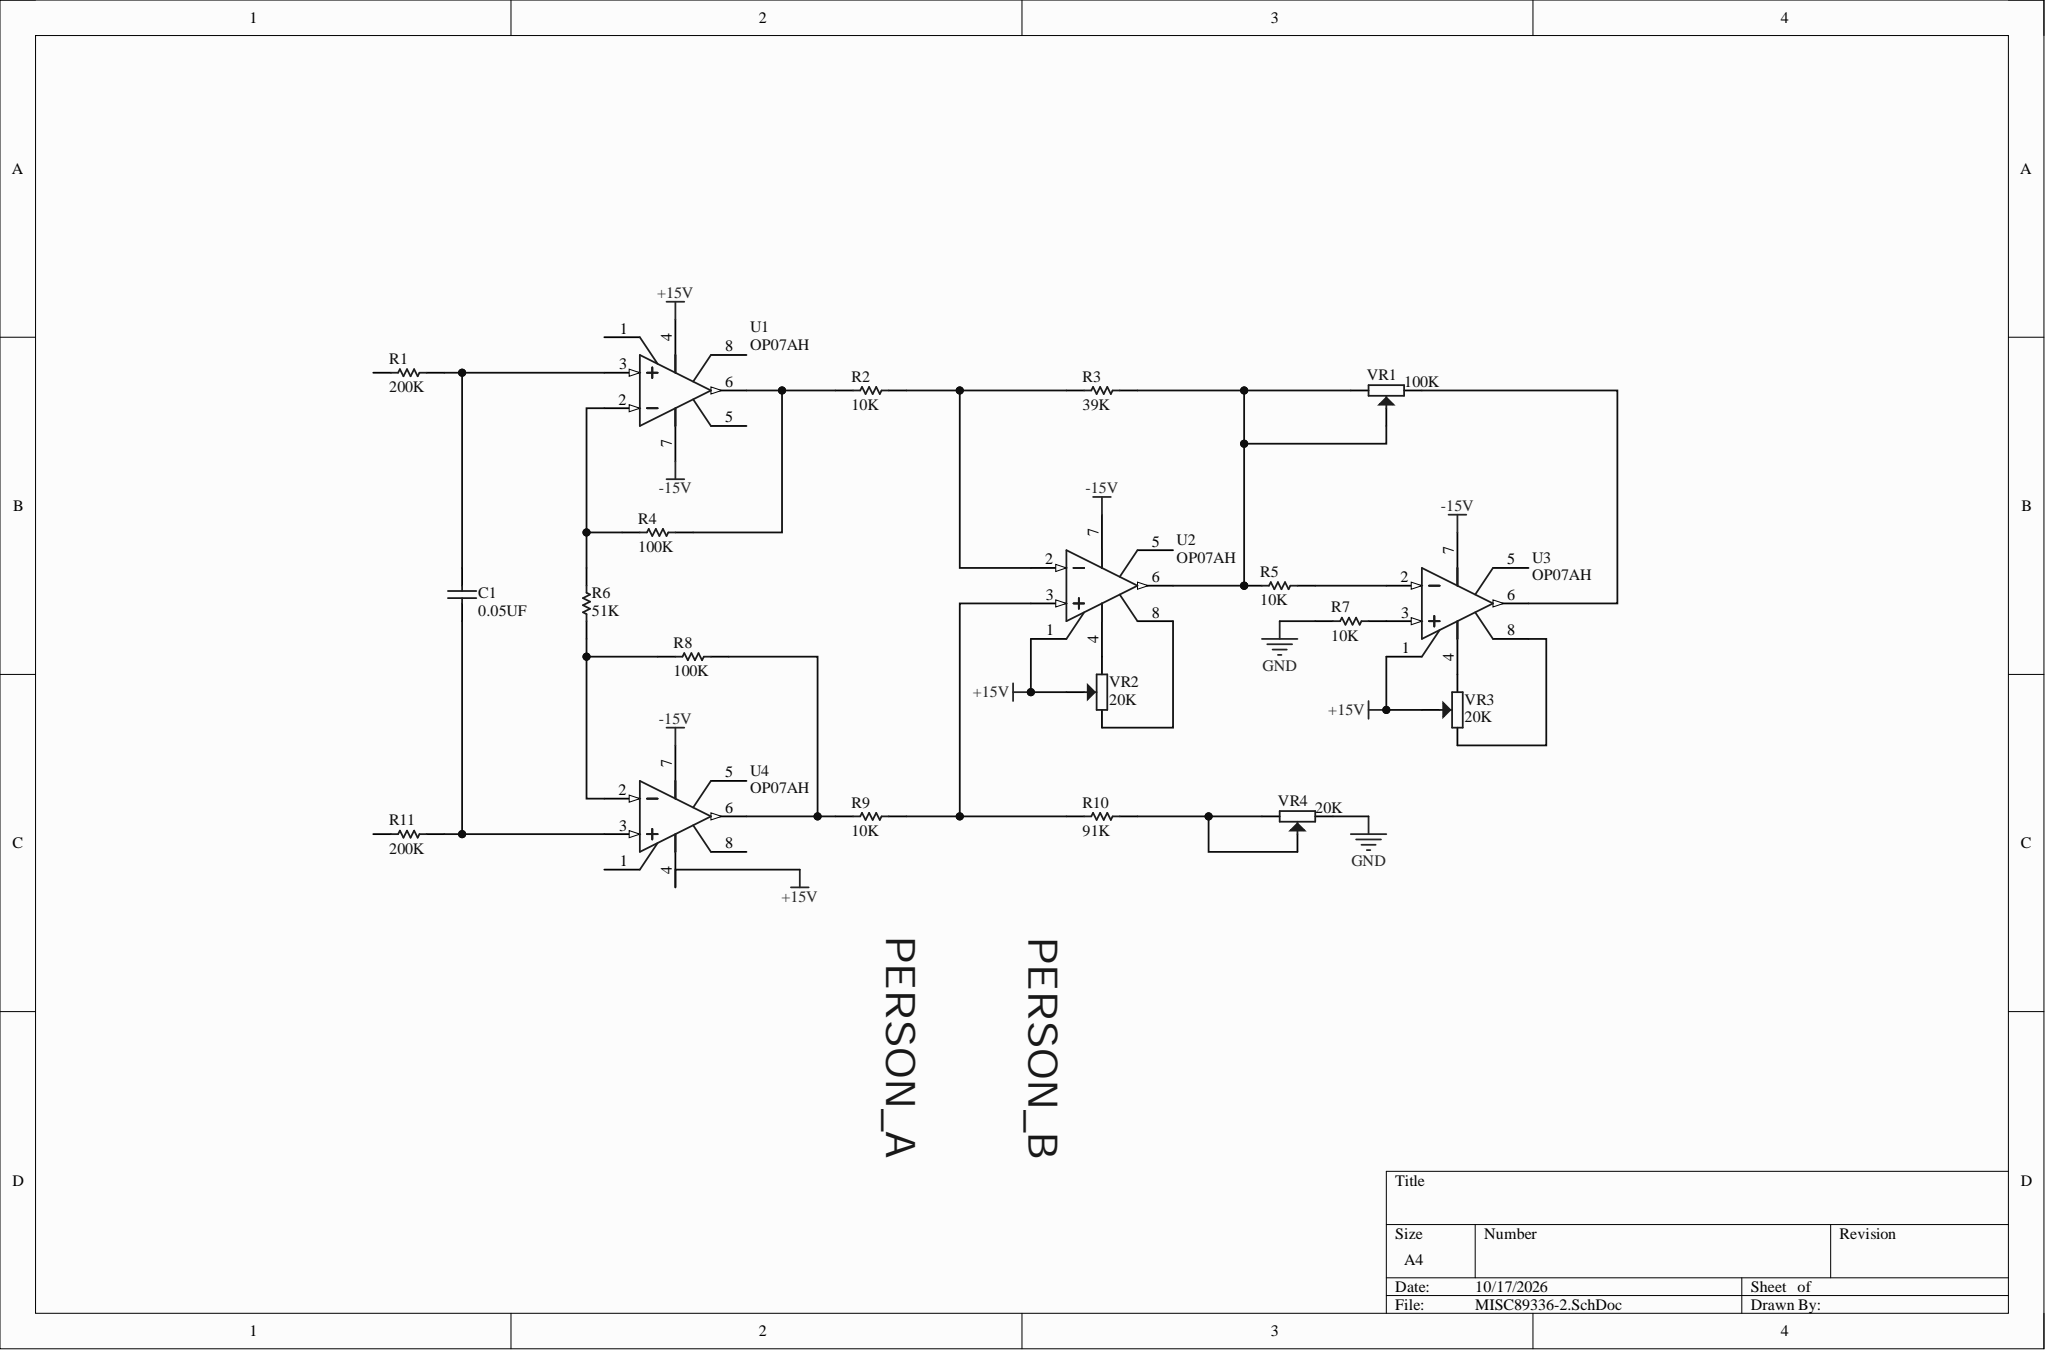Circuit board | Altium Designer | 20 parts | 20 nets
Bill of materials:
Comment,Description,Designator,Footprint,LibRef,Quantity
"0.05UF","Capacitor (Semiconductor SIM Model)","C1","C2512","Cap Semi","1"
"200K","","R1, R11","AXIAL0.4","RES","2"
"10K","","R2, R5, R7, R9","AXIAL0.4","RES","4"
"39K","","R3","AXIAL0.4","RES","1"
"100K","","R4, R8","AXIAL0.4","RES","2"
"51K","","R6","AXIAL0.4","RES","1"
"91K","","R10","AXIAL0.4","RES","1"
"OP07AH","Ultra-Low Offset Voltage Operational Amplifier","U1, U2, U3, U4","DIP8","ADOP07AH","4"
"100K","","VR1","3296W","RESVR","1"
"20K","","VR2, VR3, VR4","3296W","RESVR","3"
Netlist (Protel format):
[
C1
C2512
0.05UF



]
[
R1
AXIAL0.4
200K



]
[
R2
AXIAL0.4
10K



]
[
R3
AXIAL0.4
39K



]
[
R4
AXIAL0.4
100K



]
[
R5
AXIAL0.4
10K



]
[
R6
AXIAL0.4
51K



]
[
R7
AXIAL0.4
10K



]
[
R8
AXIAL0.4
100K



]
[
R9
AXIAL0.4
10K



]
[
R10
AXIAL0.4
91K



]
[
R11
AXIAL0.4
200K



]
[
U1
DIP8
OP07AH



]
[
U2
DIP8
OP07AH



]
[
U3
DIP8
OP07AH



]
[
U4
DIP8
OP07AH



]
[
VR1
3296W
100K



]
[
VR2
3296W
20K



]
[
VR3
3296W
20K



]
[
VR4
3296W
20K



]
(
NetU3_8
U3-8
VR3-1
)
(
NetU3_6
U3-6
VR1-1
)
(
NetU3_4
U3-4
VR3-2
)
(
NetU2_8
U2-8
VR2-1
)
(
NetU2_4
U2-4
VR2-2
)
(
NetR10_2
R10-2
VR4-2
)
(
NetR9_2
R9-2
R10-1
U2-3
)
(
NetR8_2
R8-2
R9-1
U4-6
)
(
NetR7_2
R7-2
U3-3
)
(
NetR6_1
R6-1
R8-1
U4-2
)
(
NetR5_2
R5-2
U3-2
)
(
NetR4_1
R4-1
R6-2
U1-2
)
(
NetR3_2
R3-2
R5-1
U2-6
VR1-2
)
(
NetR2_2
R2-2
R3-1
U2-2
)
(
NetR2_1
R2-1
R4-2
U1-6
)
(
NetC1_2
C1-2
R1-2
U1-3
)
(
NetC1_1
C1-1
R11-2
U4-3
)
(
GND
R7-1
VR4-1
)
(
-15V
U1-7
U2-7
U3-7
U4-7
)
(
+15V
U1-4
U2-1
U3-1
U4-4
VR2-2
VR3-2
)